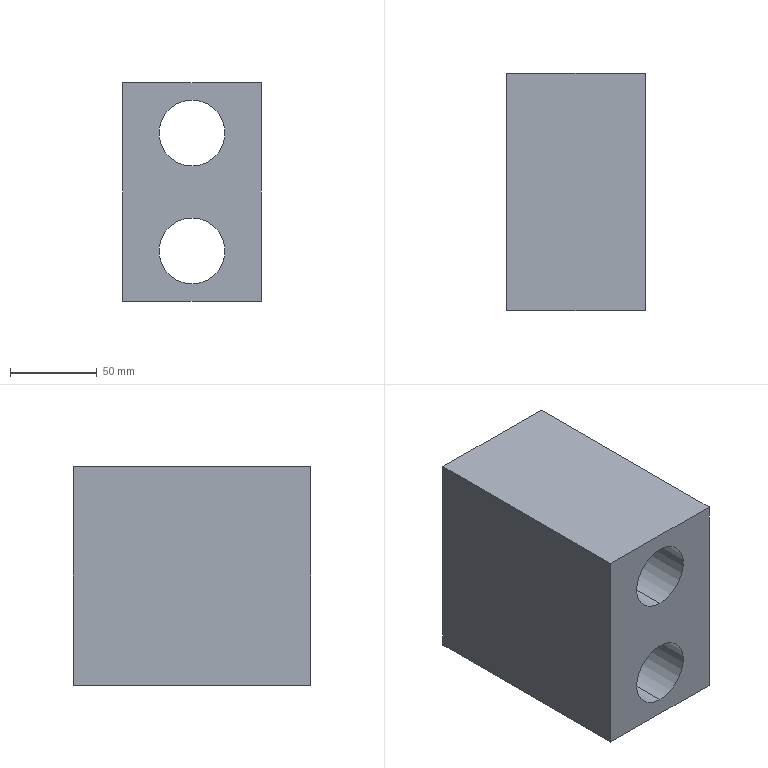Part | SolidWorks | features Extrusion 1 | 1 solid | 10 faces | box 80 x 137 x 126 mm | volume 1070213 mm3 | plane 6 | cylinder 4 | commonest cylinder face diameters 38 x4
STEP:
#1=CARTESIAN_POINT('',(0.,68.5,15.));
#2=VERTEX_POINT('',#1);
#3=CARTESIAN_POINT('',(0.,68.5,53.));
#4=VERTEX_POINT('',#3);
#5=CARTESIAN_POINT('',(0.,68.5,34.));
#6=DIRECTION('',(0.,1.,0.));
#7=DIRECTION('',(0.,0.,1.));
#8=AXIS2_PLACEMENT_3D('',#5,#6,#7);
#9=CIRCLE('',#8,19.);
#10=EDGE_CURVE('',#2,#4,#9,.T.);
#11=ORIENTED_EDGE('',*,*,#10,.T.);
#12=CARTESIAN_POINT('',(0.,-68.5,53.));
#13=VERTEX_POINT('',#12);
#14=CARTESIAN_POINT('',(0.,68.5,53.));
#15=DIRECTION('',(0.,-1.,0.));
#16=VECTOR('',#15,1000.);
#17=LINE('',#14,#16);
#18=EDGE_CURVE('',#4,#13,#17,.T.);
#19=ORIENTED_EDGE('',*,*,#18,.T.);
#20=CARTESIAN_POINT('',(0.,-68.5,15.));
#21=VERTEX_POINT('',#20);
#22=CARTESIAN_POINT('',(0.,-68.5,34.));
#23=DIRECTION('',(0.,1.,0.));
#24=DIRECTION('',(0.,0.,1.));
#25=AXIS2_PLACEMENT_3D('',#22,#23,#24);
#26=CIRCLE('',#25,19.);
#27=EDGE_CURVE('',#21,#13,#26,.T.);
#28=ORIENTED_EDGE('',*,*,#27,.F.);
#29=CARTESIAN_POINT('',(0.,68.5,15.));
#30=DIRECTION('',(0.,-1.,0.));
#31=VECTOR('',#30,1000.);
#32=LINE('',#29,#31);
#33=EDGE_CURVE('',#2,#21,#32,.T.);
#34=ORIENTED_EDGE('',*,*,#33,.F.);
#35=EDGE_LOOP('',(#11,#19,#28,#34));
#36=FACE_OUTER_BOUND('',#35,.T.);
#37=CARTESIAN_POINT('',(0.,68.5,34.));
#38=DIRECTION('',(0.,-1.,0.));
#39=DIRECTION('',(0.,0.,-1.));
#40=AXIS2_PLACEMENT_3D('',#37,#38,#39);
#41=CYLINDRICAL_SURFACE('',#40,19.);
#42=ADVANCED_FACE('',(#36),#41,.F.);
#43=CARTESIAN_POINT('',(0.,68.5,-53.));
#44=VERTEX_POINT('',#43);
#45=CARTESIAN_POINT('',(0.,68.5,-15.));
#46=VERTEX_POINT('',#45);
#47=CARTESIAN_POINT('',(0.,68.5,-34.));
#48=DIRECTION('',(0.,1.,0.));
#49=DIRECTION('',(0.,0.,1.));
#50=AXIS2_PLACEMENT_3D('',#47,#48,#49);
#51=CIRCLE('',#50,19.);
#52=EDGE_CURVE('',#44,#46,#51,.T.);
#53=ORIENTED_EDGE('',*,*,#52,.T.);
#54=CARTESIAN_POINT('',(0.,-68.5,-15.));
#55=VERTEX_POINT('',#54);
#56=CARTESIAN_POINT('',(0.,68.5,-15.));
#57=DIRECTION('',(0.,-1.,0.));
#58=VECTOR('',#57,1000.);
#59=LINE('',#56,#58);
#60=EDGE_CURVE('',#46,#55,#59,.T.);
#61=ORIENTED_EDGE('',*,*,#60,.T.);
#62=CARTESIAN_POINT('',(0.,-68.5,-53.));
#63=VERTEX_POINT('',#62);
#64=CARTESIAN_POINT('',(0.,-68.5,-34.));
#65=DIRECTION('',(0.,1.,0.));
#66=DIRECTION('',(0.,0.,1.));
#67=AXIS2_PLACEMENT_3D('',#64,#65,#66);
#68=CIRCLE('',#67,19.);
#69=EDGE_CURVE('',#63,#55,#68,.T.);
#70=ORIENTED_EDGE('',*,*,#69,.F.);
#71=CARTESIAN_POINT('',(0.,68.5,-53.));
#72=DIRECTION('',(0.,-1.,0.));
#73=VECTOR('',#72,1000.);
#74=LINE('',#71,#73);
#75=EDGE_CURVE('',#44,#63,#74,.T.);
#76=ORIENTED_EDGE('',*,*,#75,.F.);
#77=EDGE_LOOP('',(#53,#61,#70,#76));
#78=FACE_OUTER_BOUND('',#77,.T.);
#79=CARTESIAN_POINT('',(0.,68.5,-34.));
#80=DIRECTION('',(0.,-1.,0.));
#81=DIRECTION('',(0.,0.,-1.));
#82=AXIS2_PLACEMENT_3D('',#79,#80,#81);
#83=CYLINDRICAL_SURFACE('',#82,19.);
#84=ADVANCED_FACE('',(#78),#83,.F.);
#85=ORIENTED_EDGE('',*,*,#52,.F.);
#86=CARTESIAN_POINT('',(0.,68.5,-34.));
#87=DIRECTION('',(0.,1.,0.));
#88=DIRECTION('',(0.,0.,1.));
#89=AXIS2_PLACEMENT_3D('',#86,#87,#88);
#90=CIRCLE('',#89,19.);
#91=EDGE_CURVE('',#46,#44,#90,.T.);
#92=ORIENTED_EDGE('',*,*,#91,.F.);
#93=EDGE_LOOP('',(#85,#92));
#94=FACE_BOUND('',#93,.T.);
#95=CARTESIAN_POINT('',(-40.,68.5,-63.));
#96=VERTEX_POINT('',#95);
#97=CARTESIAN_POINT('',(-40.,68.5,63.));
#98=VERTEX_POINT('',#97);
#99=CARTESIAN_POINT('',(-40.,68.5,-63.));
#100=DIRECTION('',(0.,0.,1.));
#101=VECTOR('',#100,1000.);
#102=LINE('',#99,#101);
#103=EDGE_CURVE('',#96,#98,#102,.T.);
#104=ORIENTED_EDGE('',*,*,#103,.T.);
#105=CARTESIAN_POINT('',(40.,68.5,63.));
#106=VERTEX_POINT('',#105);
#107=CARTESIAN_POINT('',(-40.,68.5,63.));
#108=DIRECTION('',(1.,0.,0.));
#109=VECTOR('',#108,1000.);
#110=LINE('',#107,#109);
#111=EDGE_CURVE('',#98,#106,#110,.T.);
#112=ORIENTED_EDGE('',*,*,#111,.T.);
#113=CARTESIAN_POINT('',(40.,68.5,-63.));
#114=VERTEX_POINT('',#113);
#115=CARTESIAN_POINT('',(40.,68.5,-63.));
#116=DIRECTION('',(0.,0.,-1.));
#117=VECTOR('',#116,1000.);
#118=LINE('',#115,#117);
#119=EDGE_CURVE('',#106,#114,#118,.T.);
#120=ORIENTED_EDGE('',*,*,#119,.T.);
#121=CARTESIAN_POINT('',(-40.,68.5,-63.));
#122=DIRECTION('',(-1.,0.,0.));
#123=VECTOR('',#122,1000.);
#124=LINE('',#121,#123);
#125=EDGE_CURVE('',#114,#96,#124,.T.);
#126=ORIENTED_EDGE('',*,*,#125,.T.);
#127=EDGE_LOOP('',(#104,#112,#120,#126));
#128=FACE_OUTER_BOUND('',#127,.T.);
#129=ORIENTED_EDGE('',*,*,#10,.F.);
#130=CARTESIAN_POINT('',(0.,68.5,34.));
#131=DIRECTION('',(0.,1.,0.));
#132=DIRECTION('',(0.,0.,1.));
#133=AXIS2_PLACEMENT_3D('',#130,#131,#132);
#134=CIRCLE('',#133,19.);
#135=EDGE_CURVE('',#4,#2,#134,.T.);
#136=ORIENTED_EDGE('',*,*,#135,.F.);
#137=EDGE_LOOP('',(#129,#136));
#138=FACE_BOUND('',#137,.T.);
#139=CARTESIAN_POINT('',(0.,68.5,0.));
#140=DIRECTION('',(0.,1.,0.));
#141=DIRECTION('',(0.,0.,1.));
#142=AXIS2_PLACEMENT_3D('',#139,#140,#141);
#143=PLANE('',#142);
#144=ADVANCED_FACE('',(#94,#128,#138),#143,.T.);
#145=ORIENTED_EDGE('',*,*,#69,.T.);
#146=CARTESIAN_POINT('',(0.,-68.5,-34.));
#147=DIRECTION('',(0.,1.,0.));
#148=DIRECTION('',(0.,0.,1.));
#149=AXIS2_PLACEMENT_3D('',#146,#147,#148);
#150=CIRCLE('',#149,19.);
#151=EDGE_CURVE('',#55,#63,#150,.T.);
#152=ORIENTED_EDGE('',*,*,#151,.T.);
#153=EDGE_LOOP('',(#145,#152));
#154=FACE_BOUND('',#153,.T.);
#155=CARTESIAN_POINT('',(-40.,-68.5,-63.));
#156=VERTEX_POINT('',#155);
#157=CARTESIAN_POINT('',(-40.,-68.5,63.));
#158=VERTEX_POINT('',#157);
#159=CARTESIAN_POINT('',(-40.,-68.5,-63.));
#160=DIRECTION('',(0.,0.,1.));
#161=VECTOR('',#160,1000.);
#162=LINE('',#159,#161);
#163=EDGE_CURVE('',#156,#158,#162,.T.);
#164=ORIENTED_EDGE('',*,*,#163,.F.);
#165=CARTESIAN_POINT('',(40.,-68.5,-63.));
#166=VERTEX_POINT('',#165);
#167=CARTESIAN_POINT('',(-40.,-68.5,-63.));
#168=DIRECTION('',(-1.,0.,0.));
#169=VECTOR('',#168,1000.);
#170=LINE('',#167,#169);
#171=EDGE_CURVE('',#166,#156,#170,.T.);
#172=ORIENTED_EDGE('',*,*,#171,.F.);
#173=CARTESIAN_POINT('',(40.,-68.5,63.));
#174=VERTEX_POINT('',#173);
#175=CARTESIAN_POINT('',(40.,-68.5,-63.));
#176=DIRECTION('',(0.,0.,-1.));
#177=VECTOR('',#176,1000.);
#178=LINE('',#175,#177);
#179=EDGE_CURVE('',#174,#166,#178,.T.);
#180=ORIENTED_EDGE('',*,*,#179,.F.);
#181=CARTESIAN_POINT('',(-40.,-68.5,63.));
#182=DIRECTION('',(1.,0.,0.));
#183=VECTOR('',#182,1000.);
#184=LINE('',#181,#183);
#185=EDGE_CURVE('',#158,#174,#184,.T.);
#186=ORIENTED_EDGE('',*,*,#185,.F.);
#187=EDGE_LOOP('',(#164,#172,#180,#186));
#188=FACE_OUTER_BOUND('',#187,.T.);
#189=ORIENTED_EDGE('',*,*,#27,.T.);
#190=CARTESIAN_POINT('',(0.,-68.5,34.));
#191=DIRECTION('',(0.,1.,0.));
#192=DIRECTION('',(0.,0.,1.));
#193=AXIS2_PLACEMENT_3D('',#190,#191,#192);
#194=CIRCLE('',#193,19.);
#195=EDGE_CURVE('',#13,#21,#194,.T.);
#196=ORIENTED_EDGE('',*,*,#195,.T.);
#197=EDGE_LOOP('',(#189,#196));
#198=FACE_BOUND('',#197,.T.);
#199=CARTESIAN_POINT('',(0.,-68.5,0.));
#200=DIRECTION('',(0.,1.,0.));
#201=DIRECTION('',(0.,0.,1.));
#202=AXIS2_PLACEMENT_3D('',#199,#200,#201);
#203=PLANE('',#202);
#204=ADVANCED_FACE('',(#154,#188,#198),#203,.F.);
#205=ORIENTED_EDGE('',*,*,#163,.T.);
#206=CARTESIAN_POINT('',(-40.,68.5,63.));
#207=DIRECTION('',(0.,-1.,0.));
#208=VECTOR('',#207,1000.);
#209=LINE('',#206,#208);
#210=EDGE_CURVE('',#98,#158,#209,.T.);
#211=ORIENTED_EDGE('',*,*,#210,.F.);
#212=ORIENTED_EDGE('',*,*,#103,.F.);
#213=CARTESIAN_POINT('',(-40.,68.5,-63.));
#214=DIRECTION('',(0.,-1.,0.));
#215=VECTOR('',#214,1000.);
#216=LINE('',#213,#215);
#217=EDGE_CURVE('',#96,#156,#216,.T.);
#218=ORIENTED_EDGE('',*,*,#217,.T.);
#219=EDGE_LOOP('',(#205,#211,#212,#218));
#220=FACE_OUTER_BOUND('',#219,.T.);
#221=CARTESIAN_POINT('',(-40.,68.5,-63.));
#222=DIRECTION('',(1.,0.,0.));
#223=DIRECTION('',(0.,0.,-1.));
#224=AXIS2_PLACEMENT_3D('',#221,#222,#223);
#225=PLANE('',#224);
#226=ADVANCED_FACE('',(#220),#225,.F.);
#227=ORIENTED_EDGE('',*,*,#185,.T.);
#228=CARTESIAN_POINT('',(40.,68.5,63.));
#229=DIRECTION('',(0.,-1.,0.));
#230=VECTOR('',#229,1000.);
#231=LINE('',#228,#230);
#232=EDGE_CURVE('',#106,#174,#231,.T.);
#233=ORIENTED_EDGE('',*,*,#232,.F.);
#234=ORIENTED_EDGE('',*,*,#111,.F.);
#235=ORIENTED_EDGE('',*,*,#210,.T.);
#236=EDGE_LOOP('',(#227,#233,#234,#235));
#237=FACE_OUTER_BOUND('',#236,.T.);
#238=CARTESIAN_POINT('',(-40.,68.5,63.));
#239=DIRECTION('',(0.,0.,-1.));
#240=DIRECTION('',(-1.,0.,0.));
#241=AXIS2_PLACEMENT_3D('',#238,#239,#240);
#242=PLANE('',#241);
#243=ADVANCED_FACE('',(#237),#242,.F.);
#244=ORIENTED_EDGE('',*,*,#179,.T.);
#245=CARTESIAN_POINT('',(40.,68.5,-63.));
#246=DIRECTION('',(0.,-1.,0.));
#247=VECTOR('',#246,1000.);
#248=LINE('',#245,#247);
#249=EDGE_CURVE('',#114,#166,#248,.T.);
#250=ORIENTED_EDGE('',*,*,#249,.F.);
#251=ORIENTED_EDGE('',*,*,#119,.F.);
#252=ORIENTED_EDGE('',*,*,#232,.T.);
#253=EDGE_LOOP('',(#244,#250,#251,#252));
#254=FACE_OUTER_BOUND('',#253,.T.);
#255=CARTESIAN_POINT('',(40.,68.5,-63.));
#256=DIRECTION('',(-1.,0.,0.));
#257=DIRECTION('',(0.,0.,1.));
#258=AXIS2_PLACEMENT_3D('',#255,#256,#257);
#259=PLANE('',#258);
#260=ADVANCED_FACE('',(#254),#259,.F.);
#261=ORIENTED_EDGE('',*,*,#171,.T.);
#262=ORIENTED_EDGE('',*,*,#217,.F.);
#263=ORIENTED_EDGE('',*,*,#125,.F.);
#264=ORIENTED_EDGE('',*,*,#249,.T.);
#265=EDGE_LOOP('',(#261,#262,#263,#264));
#266=FACE_OUTER_BOUND('',#265,.T.);
#267=CARTESIAN_POINT('',(-40.,68.5,-63.));
#268=DIRECTION('',(0.,0.,1.));
#269=DIRECTION('',(1.,0.,0.));
#270=AXIS2_PLACEMENT_3D('',#267,#268,#269);
#271=PLANE('',#270);
#272=ADVANCED_FACE('',(#266),#271,.F.);
#273=ORIENTED_EDGE('',*,*,#60,.F.);
#274=ORIENTED_EDGE('',*,*,#91,.T.);
#275=ORIENTED_EDGE('',*,*,#75,.T.);
#276=ORIENTED_EDGE('',*,*,#151,.F.);
#277=EDGE_LOOP('',(#273,#274,#275,#276));
#278=FACE_OUTER_BOUND('',#277,.T.);
#279=CARTESIAN_POINT('',(0.,68.5,-34.));
#280=DIRECTION('',(0.,-1.,0.));
#281=DIRECTION('',(0.,0.,-1.));
#282=AXIS2_PLACEMENT_3D('',#279,#280,#281);
#283=CYLINDRICAL_SURFACE('',#282,19.);
#284=ADVANCED_FACE('',(#278),#283,.F.);
#285=ORIENTED_EDGE('',*,*,#18,.F.);
#286=ORIENTED_EDGE('',*,*,#135,.T.);
#287=ORIENTED_EDGE('',*,*,#33,.T.);
#288=ORIENTED_EDGE('',*,*,#195,.F.);
#289=EDGE_LOOP('',(#285,#286,#287,#288));
#290=FACE_OUTER_BOUND('',#289,.T.);
#291=CARTESIAN_POINT('',(0.,68.5,34.));
#292=DIRECTION('',(0.,-1.,0.));
#293=DIRECTION('',(0.,0.,-1.));
#294=AXIS2_PLACEMENT_3D('',#291,#292,#293);
#295=CYLINDRICAL_SURFACE('',#294,19.);
#296=ADVANCED_FACE('',(#290),#295,.F.);
#297=CLOSED_SHELL('',(#42,#84,#144,#204,#226,#243,#260,#272,#284,#296));
#298=MANIFOLD_SOLID_BREP('',#297);
#299=CARTESIAN_POINT('',(0.,0.,0.));
#300=DIRECTION('',(0.,0.,1.));
#301=DIRECTION('',(1.,0.,0.));
#302=AXIS2_PLACEMENT_3D('',#299,#300,#301);
#303=(LENGTH_UNIT()NAMED_UNIT(*)SI_UNIT(.MILLI.,.METRE.));
#304=UNCERTAINTY_MEASURE_WITH_UNIT(LENGTH_MEASURE(0.00001),#303,'','');
#305=(NAMED_UNIT(*)PLANE_ANGLE_UNIT()SI_UNIT($,.RADIAN.));
#306=(NAMED_UNIT(*)SI_UNIT($,.STERADIAN.)SOLID_ANGLE_UNIT());
#307=(GEOMETRIC_REPRESENTATION_CONTEXT(3)GLOBAL_UNCERTAINTY_ASSIGNED_CONTEXT((#304))GLOBAL_UNIT_ASSIGNED_CONTEXT((#303,#305,#306))REPRESENTATION_CONTEXT('',''));
#308=ADVANCED_BREP_SHAPE_REPRESENTATION('',(#298,#302),#307);